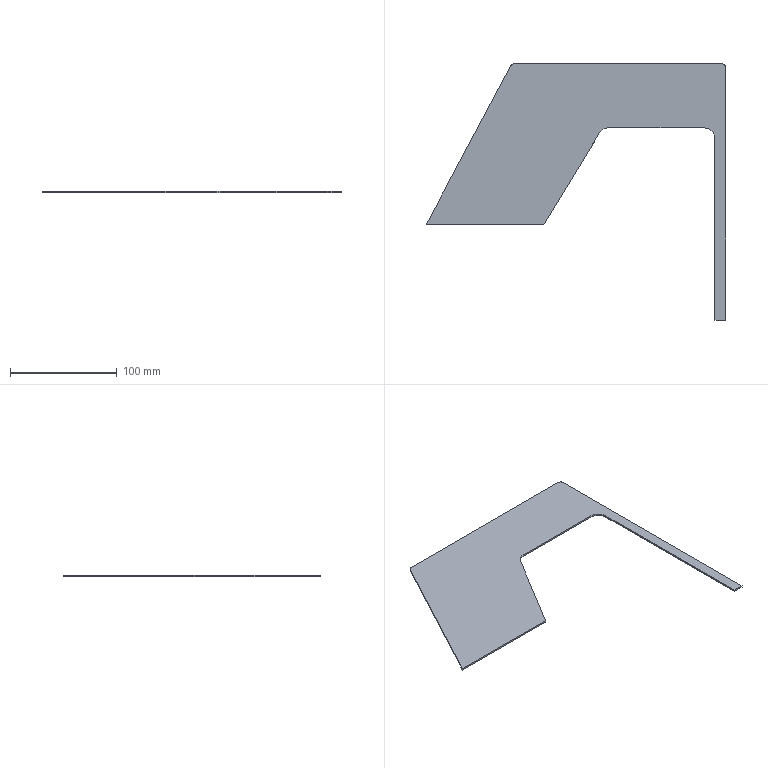Part | SolidWorks | features Extrusion 1 | 1 solid | 14 faces | box 280 x 240 x 1.5 mm | volume 37497 mm3 | plane 10 | cylinder 4 | commonest cylinder face diameters 7 x2 20 x2
STEP:
#1=CARTESIAN_POINT('',(162.076,85.215,0.));
#2=VERTEX_POINT('',#1);
#3=CARTESIAN_POINT('',(110.,0.,0.));
#4=VERTEX_POINT('',#3);
#5=CARTESIAN_POINT('',(162.076,85.215,0.));
#6=DIRECTION('',(-0.5215,-0.8533,0.));
#7=VECTOR('',#6,1000.);
#8=LINE('',#5,#7);
#9=EDGE_CURVE('',#2,#4,#8,.T.);
#10=ORIENTED_EDGE('',*,*,#9,.F.);
#11=CARTESIAN_POINT('',(162.076,85.215,1.5));
#12=VERTEX_POINT('',#11);
#13=CARTESIAN_POINT('',(162.076,85.215,1.5));
#14=DIRECTION('',(0.,0.,-1.));
#15=VECTOR('',#14,1000.);
#16=LINE('',#13,#15);
#17=EDGE_CURVE('',#12,#2,#16,.T.);
#18=ORIENTED_EDGE('',*,*,#17,.F.);
#19=CARTESIAN_POINT('',(110.,0.,1.5));
#20=VERTEX_POINT('',#19);
#21=CARTESIAN_POINT('',(162.076,85.215,1.5));
#22=DIRECTION('',(-0.5215,-0.8533,0.));
#23=VECTOR('',#22,1000.);
#24=LINE('',#21,#23);
#25=EDGE_CURVE('',#12,#20,#24,.T.);
#26=ORIENTED_EDGE('',*,*,#25,.T.);
#27=CARTESIAN_POINT('',(110.,0.,1.5));
#28=DIRECTION('',(0.,0.,-1.));
#29=VECTOR('',#28,1000.);
#30=LINE('',#27,#29);
#31=EDGE_CURVE('',#20,#4,#30,.T.);
#32=ORIENTED_EDGE('',*,*,#31,.T.);
#33=EDGE_LOOP('',(#10,#18,#26,#32));
#34=FACE_OUTER_BOUND('',#33,.T.);
#35=CARTESIAN_POINT('',(162.076,85.215,1.5));
#36=DIRECTION('',(0.8533,-0.5215,0.));
#37=DIRECTION('',(0.5215,0.8533,0.));
#38=AXIS2_PLACEMENT_3D('',#35,#36,#37);
#39=PLANE('',#38);
#40=ADVANCED_FACE('',(#34),#39,.T.);
#41=CARTESIAN_POINT('',(170.608,90.,0.));
#42=VERTEX_POINT('',#41);
#43=CARTESIAN_POINT('',(170.608,80.,0.));
#44=DIRECTION('',(0.,0.,1.));
#45=DIRECTION('',(1.,0.,0.));
#46=AXIS2_PLACEMENT_3D('',#43,#44,#45);
#47=CIRCLE('',#46,10.);
#48=EDGE_CURVE('',#42,#2,#47,.T.);
#49=ORIENTED_EDGE('',*,*,#48,.F.);
#50=CARTESIAN_POINT('',(170.608,90.,1.5));
#51=VERTEX_POINT('',#50);
#52=CARTESIAN_POINT('',(170.608,90.,1.5));
#53=DIRECTION('',(0.,0.,-1.));
#54=VECTOR('',#53,1000.);
#55=LINE('',#52,#54);
#56=EDGE_CURVE('',#51,#42,#55,.T.);
#57=ORIENTED_EDGE('',*,*,#56,.F.);
#58=CARTESIAN_POINT('',(170.608,80.,1.5));
#59=DIRECTION('',(0.,0.,1.));
#60=DIRECTION('',(1.,0.,0.));
#61=AXIS2_PLACEMENT_3D('',#58,#59,#60);
#62=CIRCLE('',#61,10.);
#63=EDGE_CURVE('',#51,#12,#62,.T.);
#64=ORIENTED_EDGE('',*,*,#63,.T.);
#65=ORIENTED_EDGE('',*,*,#17,.T.);
#66=EDGE_LOOP('',(#49,#57,#64,#65));
#67=FACE_OUTER_BOUND('',#66,.T.);
#68=CARTESIAN_POINT('',(170.608,80.,1.5));
#69=DIRECTION('',(0.,0.,-1.));
#70=DIRECTION('',(-1.,0.,0.));
#71=AXIS2_PLACEMENT_3D('',#68,#69,#70);
#72=CYLINDRICAL_SURFACE('',#71,10.);
#73=ADVANCED_FACE('',(#67),#72,.F.);
#74=CARTESIAN_POINT('',(260.,90.,0.));
#75=VERTEX_POINT('',#74);
#76=CARTESIAN_POINT('',(260.,90.,0.));
#77=DIRECTION('',(-1.,0.,0.));
#78=VECTOR('',#77,1000.);
#79=LINE('',#76,#78);
#80=EDGE_CURVE('',#75,#42,#79,.T.);
#81=ORIENTED_EDGE('',*,*,#80,.F.);
#82=CARTESIAN_POINT('',(260.,90.,1.5));
#83=VERTEX_POINT('',#82);
#84=CARTESIAN_POINT('',(260.,90.,1.5));
#85=DIRECTION('',(0.,0.,-1.));
#86=VECTOR('',#85,1000.);
#87=LINE('',#84,#86);
#88=EDGE_CURVE('',#83,#75,#87,.T.);
#89=ORIENTED_EDGE('',*,*,#88,.F.);
#90=CARTESIAN_POINT('',(260.,90.,1.5));
#91=DIRECTION('',(-1.,0.,0.));
#92=VECTOR('',#91,1000.);
#93=LINE('',#90,#92);
#94=EDGE_CURVE('',#83,#51,#93,.T.);
#95=ORIENTED_EDGE('',*,*,#94,.T.);
#96=ORIENTED_EDGE('',*,*,#56,.T.);
#97=EDGE_LOOP('',(#81,#89,#95,#96));
#98=FACE_OUTER_BOUND('',#97,.T.);
#99=CARTESIAN_POINT('',(260.,90.,1.5));
#100=DIRECTION('',(0.,-1.,0.));
#101=DIRECTION('',(0.,0.,-1.));
#102=AXIS2_PLACEMENT_3D('',#99,#100,#101);
#103=PLANE('',#102);
#104=ADVANCED_FACE('',(#98),#103,.T.);
#105=CARTESIAN_POINT('',(270.,80.,0.));
#106=VERTEX_POINT('',#105);
#107=CARTESIAN_POINT('',(260.,80.,0.));
#108=DIRECTION('',(0.,0.,1.));
#109=DIRECTION('',(1.,0.,0.));
#110=AXIS2_PLACEMENT_3D('',#107,#108,#109);
#111=CIRCLE('',#110,10.);
#112=EDGE_CURVE('',#106,#75,#111,.T.);
#113=ORIENTED_EDGE('',*,*,#112,.F.);
#114=CARTESIAN_POINT('',(270.,80.,1.5));
#115=VERTEX_POINT('',#114);
#116=CARTESIAN_POINT('',(270.,80.,1.5));
#117=DIRECTION('',(0.,0.,-1.));
#118=VECTOR('',#117,1000.);
#119=LINE('',#116,#118);
#120=EDGE_CURVE('',#115,#106,#119,.T.);
#121=ORIENTED_EDGE('',*,*,#120,.F.);
#122=CARTESIAN_POINT('',(260.,80.,1.5));
#123=DIRECTION('',(0.,0.,1.));
#124=DIRECTION('',(1.,0.,0.));
#125=AXIS2_PLACEMENT_3D('',#122,#123,#124);
#126=CIRCLE('',#125,10.);
#127=EDGE_CURVE('',#115,#83,#126,.T.);
#128=ORIENTED_EDGE('',*,*,#127,.T.);
#129=ORIENTED_EDGE('',*,*,#88,.T.);
#130=EDGE_LOOP('',(#113,#121,#128,#129));
#131=FACE_OUTER_BOUND('',#130,.T.);
#132=CARTESIAN_POINT('',(260.,80.,1.5));
#133=DIRECTION('',(0.,0.,-1.));
#134=DIRECTION('',(-1.,0.,0.));
#135=AXIS2_PLACEMENT_3D('',#132,#133,#134);
#136=CYLINDRICAL_SURFACE('',#135,10.);
#137=ADVANCED_FACE('',(#131),#136,.F.);
#138=CARTESIAN_POINT('',(270.,-90.,0.));
#139=VERTEX_POINT('',#138);
#140=CARTESIAN_POINT('',(270.,-90.,0.));
#141=DIRECTION('',(0.,1.,0.));
#142=VECTOR('',#141,1000.);
#143=LINE('',#140,#142);
#144=EDGE_CURVE('',#139,#106,#143,.T.);
#145=ORIENTED_EDGE('',*,*,#144,.F.);
#146=CARTESIAN_POINT('',(270.,-90.,1.5));
#147=VERTEX_POINT('',#146);
#148=CARTESIAN_POINT('',(270.,-90.,1.5));
#149=DIRECTION('',(0.,0.,-1.));
#150=VECTOR('',#149,1000.);
#151=LINE('',#148,#150);
#152=EDGE_CURVE('',#147,#139,#151,.T.);
#153=ORIENTED_EDGE('',*,*,#152,.F.);
#154=CARTESIAN_POINT('',(270.,-90.,1.5));
#155=DIRECTION('',(0.,1.,0.));
#156=VECTOR('',#155,1000.);
#157=LINE('',#154,#156);
#158=EDGE_CURVE('',#147,#115,#157,.T.);
#159=ORIENTED_EDGE('',*,*,#158,.T.);
#160=ORIENTED_EDGE('',*,*,#120,.T.);
#161=EDGE_LOOP('',(#145,#153,#159,#160));
#162=FACE_OUTER_BOUND('',#161,.T.);
#163=CARTESIAN_POINT('',(270.,-90.,1.5));
#164=DIRECTION('',(-1.,0.,0.));
#165=DIRECTION('',(0.,-1.,0.));
#166=AXIS2_PLACEMENT_3D('',#163,#164,#165);
#167=PLANE('',#166);
#168=ADVANCED_FACE('',(#162),#167,.T.);
#169=CARTESIAN_POINT('',(280.,-90.,0.));
#170=VERTEX_POINT('',#169);
#171=CARTESIAN_POINT('',(280.,-90.,0.));
#172=DIRECTION('',(-1.,0.,0.));
#173=VECTOR('',#172,1000.);
#174=LINE('',#171,#173);
#175=EDGE_CURVE('',#170,#139,#174,.T.);
#176=ORIENTED_EDGE('',*,*,#175,.F.);
#177=CARTESIAN_POINT('',(280.,-90.,1.5));
#178=VERTEX_POINT('',#177);
#179=CARTESIAN_POINT('',(280.,-90.,1.5));
#180=DIRECTION('',(0.,0.,-1.));
#181=VECTOR('',#180,1000.);
#182=LINE('',#179,#181);
#183=EDGE_CURVE('',#178,#170,#182,.T.);
#184=ORIENTED_EDGE('',*,*,#183,.F.);
#185=CARTESIAN_POINT('',(280.,-90.,1.5));
#186=DIRECTION('',(-1.,0.,0.));
#187=VECTOR('',#186,1000.);
#188=LINE('',#185,#187);
#189=EDGE_CURVE('',#178,#147,#188,.T.);
#190=ORIENTED_EDGE('',*,*,#189,.T.);
#191=ORIENTED_EDGE('',*,*,#152,.T.);
#192=EDGE_LOOP('',(#176,#184,#190,#191));
#193=FACE_OUTER_BOUND('',#192,.T.);
#194=CARTESIAN_POINT('',(280.,-90.,1.5));
#195=DIRECTION('',(0.,-1.,0.));
#196=DIRECTION('',(0.,0.,-1.));
#197=AXIS2_PLACEMENT_3D('',#194,#195,#196);
#198=PLANE('',#197);
#199=ADVANCED_FACE('',(#193),#198,.T.);
#200=CARTESIAN_POINT('',(280.,146.5,0.));
#201=VERTEX_POINT('',#200);
#202=CARTESIAN_POINT('',(280.,146.5,0.));
#203=DIRECTION('',(0.,-1.,0.));
#204=VECTOR('',#203,1000.);
#205=LINE('',#202,#204);
#206=EDGE_CURVE('',#201,#170,#205,.T.);
#207=ORIENTED_EDGE('',*,*,#206,.F.);
#208=CARTESIAN_POINT('',(280.,146.5,1.5));
#209=VERTEX_POINT('',#208);
#210=CARTESIAN_POINT('',(280.,146.5,1.5));
#211=DIRECTION('',(0.,0.,-1.));
#212=VECTOR('',#211,1000.);
#213=LINE('',#210,#212);
#214=EDGE_CURVE('',#209,#201,#213,.T.);
#215=ORIENTED_EDGE('',*,*,#214,.F.);
#216=CARTESIAN_POINT('',(280.,146.5,1.5));
#217=DIRECTION('',(0.,-1.,0.));
#218=VECTOR('',#217,1000.);
#219=LINE('',#216,#218);
#220=EDGE_CURVE('',#209,#178,#219,.T.);
#221=ORIENTED_EDGE('',*,*,#220,.T.);
#222=ORIENTED_EDGE('',*,*,#183,.T.);
#223=EDGE_LOOP('',(#207,#215,#221,#222));
#224=FACE_OUTER_BOUND('',#223,.T.);
#225=CARTESIAN_POINT('',(280.,146.5,1.5));
#226=DIRECTION('',(1.,0.,0.));
#227=DIRECTION('',(0.,0.,-1.));
#228=AXIS2_PLACEMENT_3D('',#225,#226,#227);
#229=PLANE('',#228);
#230=ADVANCED_FACE('',(#224),#229,.T.);
#231=CARTESIAN_POINT('',(276.5,150.,0.));
#232=VERTEX_POINT('',#231);
#233=CARTESIAN_POINT('',(276.5,146.5,0.));
#234=DIRECTION('',(0.,0.,-1.));
#235=DIRECTION('',(-1.,0.,0.));
#236=AXIS2_PLACEMENT_3D('',#233,#234,#235);
#237=CIRCLE('',#236,3.5);
#238=EDGE_CURVE('',#232,#201,#237,.T.);
#239=ORIENTED_EDGE('',*,*,#238,.F.);
#240=CARTESIAN_POINT('',(276.5,150.,1.5));
#241=VERTEX_POINT('',#240);
#242=CARTESIAN_POINT('',(276.5,150.,1.5));
#243=DIRECTION('',(0.,0.,-1.));
#244=VECTOR('',#243,1000.);
#245=LINE('',#242,#244);
#246=EDGE_CURVE('',#241,#232,#245,.T.);
#247=ORIENTED_EDGE('',*,*,#246,.F.);
#248=CARTESIAN_POINT('',(276.5,146.5,1.5));
#249=DIRECTION('',(0.,0.,-1.));
#250=DIRECTION('',(-1.,0.,0.));
#251=AXIS2_PLACEMENT_3D('',#248,#249,#250);
#252=CIRCLE('',#251,3.5);
#253=EDGE_CURVE('',#241,#209,#252,.T.);
#254=ORIENTED_EDGE('',*,*,#253,.T.);
#255=ORIENTED_EDGE('',*,*,#214,.T.);
#256=EDGE_LOOP('',(#239,#247,#254,#255));
#257=FACE_OUTER_BOUND('',#256,.T.);
#258=CARTESIAN_POINT('',(276.5,146.5,1.5));
#259=DIRECTION('',(0.,0.,-1.));
#260=DIRECTION('',(-1.,0.,0.));
#261=AXIS2_PLACEMENT_3D('',#258,#259,#260);
#262=CYLINDRICAL_SURFACE('',#261,3.5);
#263=ADVANCED_FACE('',(#257),#262,.T.);
#264=CARTESIAN_POINT('',(82.1,150.,0.));
#265=VERTEX_POINT('',#264);
#266=CARTESIAN_POINT('',(82.1,150.,0.));
#267=DIRECTION('',(1.,0.,0.));
#268=VECTOR('',#267,1000.);
#269=LINE('',#266,#268);
#270=EDGE_CURVE('',#265,#232,#269,.T.);
#271=ORIENTED_EDGE('',*,*,#270,.F.);
#272=CARTESIAN_POINT('',(82.1,150.,1.5));
#273=VERTEX_POINT('',#272);
#274=CARTESIAN_POINT('',(82.1,150.,1.5));
#275=DIRECTION('',(0.,0.,-1.));
#276=VECTOR('',#275,1000.);
#277=LINE('',#274,#276);
#278=EDGE_CURVE('',#273,#265,#277,.T.);
#279=ORIENTED_EDGE('',*,*,#278,.F.);
#280=CARTESIAN_POINT('',(82.1,150.,1.5));
#281=DIRECTION('',(1.,0.,0.));
#282=VECTOR('',#281,1000.);
#283=LINE('',#280,#282);
#284=EDGE_CURVE('',#273,#241,#283,.T.);
#285=ORIENTED_EDGE('',*,*,#284,.T.);
#286=ORIENTED_EDGE('',*,*,#246,.T.);
#287=EDGE_LOOP('',(#271,#279,#285,#286));
#288=FACE_OUTER_BOUND('',#287,.T.);
#289=CARTESIAN_POINT('',(82.1,150.,1.5));
#290=DIRECTION('',(0.,1.,0.));
#291=DIRECTION('',(-1.,0.,0.));
#292=AXIS2_PLACEMENT_3D('',#289,#290,#291);
#293=PLANE('',#292);
#294=ADVANCED_FACE('',(#288),#293,.T.);
#295=CARTESIAN_POINT('',(79.012,148.147,0.));
#296=VERTEX_POINT('',#295);
#297=CARTESIAN_POINT('',(82.1,146.5,0.));
#298=DIRECTION('',(0.,0.,-1.));
#299=DIRECTION('',(-1.,0.,0.));
#300=AXIS2_PLACEMENT_3D('',#297,#298,#299);
#301=CIRCLE('',#300,3.5);
#302=EDGE_CURVE('',#296,#265,#301,.T.);
#303=ORIENTED_EDGE('',*,*,#302,.F.);
#304=CARTESIAN_POINT('',(79.012,148.147,1.5));
#305=VERTEX_POINT('',#304);
#306=CARTESIAN_POINT('',(79.012,148.147,1.5));
#307=DIRECTION('',(0.,0.,-1.));
#308=VECTOR('',#307,1000.);
#309=LINE('',#306,#308);
#310=EDGE_CURVE('',#305,#296,#309,.T.);
#311=ORIENTED_EDGE('',*,*,#310,.F.);
#312=CARTESIAN_POINT('',(82.1,146.5,1.5));
#313=DIRECTION('',(0.,0.,-1.));
#314=DIRECTION('',(-1.,0.,0.));
#315=AXIS2_PLACEMENT_3D('',#312,#313,#314);
#316=CIRCLE('',#315,3.5);
#317=EDGE_CURVE('',#305,#273,#316,.T.);
#318=ORIENTED_EDGE('',*,*,#317,.T.);
#319=ORIENTED_EDGE('',*,*,#278,.T.);
#320=EDGE_LOOP('',(#303,#311,#318,#319));
#321=FACE_OUTER_BOUND('',#320,.T.);
#322=CARTESIAN_POINT('',(82.1,146.5,1.5));
#323=DIRECTION('',(0.,0.,-1.));
#324=DIRECTION('',(-1.,0.,0.));
#325=AXIS2_PLACEMENT_3D('',#322,#323,#324);
#326=CYLINDRICAL_SURFACE('',#325,3.5);
#327=ADVANCED_FACE('',(#321),#326,.T.);
#328=CARTESIAN_POINT('',(0.,0.,0.));
#329=VERTEX_POINT('',#328);
#330=CARTESIAN_POINT('',(0.,0.,0.));
#331=DIRECTION('',(0.4706,0.8824,0.));
#332=VECTOR('',#331,1000.);
#333=LINE('',#330,#332);
#334=EDGE_CURVE('',#329,#296,#333,.T.);
#335=ORIENTED_EDGE('',*,*,#334,.F.);
#336=CARTESIAN_POINT('',(0.,0.,1.5));
#337=VERTEX_POINT('',#336);
#338=CARTESIAN_POINT('',(0.,0.,1.5));
#339=DIRECTION('',(0.,0.,-1.));
#340=VECTOR('',#339,1000.);
#341=LINE('',#338,#340);
#342=EDGE_CURVE('',#337,#329,#341,.T.);
#343=ORIENTED_EDGE('',*,*,#342,.F.);
#344=CARTESIAN_POINT('',(0.,0.,1.5));
#345=DIRECTION('',(0.4706,0.8824,0.));
#346=VECTOR('',#345,1000.);
#347=LINE('',#344,#346);
#348=EDGE_CURVE('',#337,#305,#347,.T.);
#349=ORIENTED_EDGE('',*,*,#348,.T.);
#350=ORIENTED_EDGE('',*,*,#310,.T.);
#351=EDGE_LOOP('',(#335,#343,#349,#350));
#352=FACE_OUTER_BOUND('',#351,.T.);
#353=CARTESIAN_POINT('',(0.,0.,1.5));
#354=DIRECTION('',(-0.8824,0.4706,0.));
#355=DIRECTION('',(-0.4706,-0.8824,0.));
#356=AXIS2_PLACEMENT_3D('',#353,#354,#355);
#357=PLANE('',#356);
#358=ADVANCED_FACE('',(#352),#357,.T.);
#359=CARTESIAN_POINT('',(110.,0.,0.));
#360=DIRECTION('',(-1.,0.,0.));
#361=VECTOR('',#360,1000.);
#362=LINE('',#359,#361);
#363=EDGE_CURVE('',#4,#329,#362,.T.);
#364=ORIENTED_EDGE('',*,*,#363,.F.);
#365=ORIENTED_EDGE('',*,*,#31,.F.);
#366=CARTESIAN_POINT('',(110.,0.,1.5));
#367=DIRECTION('',(-1.,0.,0.));
#368=VECTOR('',#367,1000.);
#369=LINE('',#366,#368);
#370=EDGE_CURVE('',#20,#337,#369,.T.);
#371=ORIENTED_EDGE('',*,*,#370,.T.);
#372=ORIENTED_EDGE('',*,*,#342,.T.);
#373=EDGE_LOOP('',(#364,#365,#371,#372));
#374=FACE_OUTER_BOUND('',#373,.T.);
#375=CARTESIAN_POINT('',(110.,0.,1.5));
#376=DIRECTION('',(0.,-1.,0.));
#377=DIRECTION('',(0.,0.,-1.));
#378=AXIS2_PLACEMENT_3D('',#375,#376,#377);
#379=PLANE('',#378);
#380=ADVANCED_FACE('',(#374),#379,.T.);
#381=ORIENTED_EDGE('',*,*,#25,.F.);
#382=ORIENTED_EDGE('',*,*,#63,.F.);
#383=ORIENTED_EDGE('',*,*,#94,.F.);
#384=ORIENTED_EDGE('',*,*,#127,.F.);
#385=ORIENTED_EDGE('',*,*,#158,.F.);
#386=ORIENTED_EDGE('',*,*,#189,.F.);
#387=ORIENTED_EDGE('',*,*,#220,.F.);
#388=ORIENTED_EDGE('',*,*,#253,.F.);
#389=ORIENTED_EDGE('',*,*,#284,.F.);
#390=ORIENTED_EDGE('',*,*,#317,.F.);
#391=ORIENTED_EDGE('',*,*,#348,.F.);
#392=ORIENTED_EDGE('',*,*,#370,.F.);
#393=EDGE_LOOP('',(#381,#382,#383,#384,#385,#386,#387,#388,#389,#390,#391,#392));
#394=FACE_OUTER_BOUND('',#393,.T.);
#395=CARTESIAN_POINT('',(82.1,146.5,1.5));
#396=DIRECTION('',(0.,0.,-1.));
#397=DIRECTION('',(-1.,0.,0.));
#398=AXIS2_PLACEMENT_3D('',#395,#396,#397);
#399=PLANE('',#398);
#400=ADVANCED_FACE('',(#394),#399,.F.);
#401=ORIENTED_EDGE('',*,*,#9,.T.);
#402=ORIENTED_EDGE('',*,*,#363,.T.);
#403=ORIENTED_EDGE('',*,*,#334,.T.);
#404=ORIENTED_EDGE('',*,*,#302,.T.);
#405=ORIENTED_EDGE('',*,*,#270,.T.);
#406=ORIENTED_EDGE('',*,*,#238,.T.);
#407=ORIENTED_EDGE('',*,*,#206,.T.);
#408=ORIENTED_EDGE('',*,*,#175,.T.);
#409=ORIENTED_EDGE('',*,*,#144,.T.);
#410=ORIENTED_EDGE('',*,*,#112,.T.);
#411=ORIENTED_EDGE('',*,*,#80,.T.);
#412=ORIENTED_EDGE('',*,*,#48,.T.);
#413=EDGE_LOOP('',(#401,#402,#403,#404,#405,#406,#407,#408,#409,#410,#411,#412));
#414=FACE_OUTER_BOUND('',#413,.T.);
#415=CARTESIAN_POINT('',(82.1,146.5,0.));
#416=DIRECTION('',(0.,0.,-1.));
#417=DIRECTION('',(-1.,0.,0.));
#418=AXIS2_PLACEMENT_3D('',#415,#416,#417);
#419=PLANE('',#418);
#420=ADVANCED_FACE('',(#414),#419,.T.);
#421=CLOSED_SHELL('',(#40,#73,#104,#137,#168,#199,#230,#263,#294,#327,#358,#380,#400,#420));
#422=MANIFOLD_SOLID_BREP('',#421);
#423=CARTESIAN_POINT('',(0.,0.,0.));
#424=DIRECTION('',(0.,0.,1.));
#425=DIRECTION('',(1.,0.,0.));
#426=AXIS2_PLACEMENT_3D('',#423,#424,#425);
#427=(LENGTH_UNIT()NAMED_UNIT(*)SI_UNIT(.MILLI.,.METRE.));
#428=UNCERTAINTY_MEASURE_WITH_UNIT(LENGTH_MEASURE(0.00001),#427,'','');
#429=(NAMED_UNIT(*)PLANE_ANGLE_UNIT()SI_UNIT($,.RADIAN.));
#430=(NAMED_UNIT(*)SI_UNIT($,.STERADIAN.)SOLID_ANGLE_UNIT());
#431=(GEOMETRIC_REPRESENTATION_CONTEXT(3)GLOBAL_UNCERTAINTY_ASSIGNED_CONTEXT((#428))GLOBAL_UNIT_ASSIGNED_CONTEXT((#427,#429,#430))REPRESENTATION_CONTEXT('',''));
#432=ADVANCED_BREP_SHAPE_REPRESENTATION('',(#422,#426),#431);